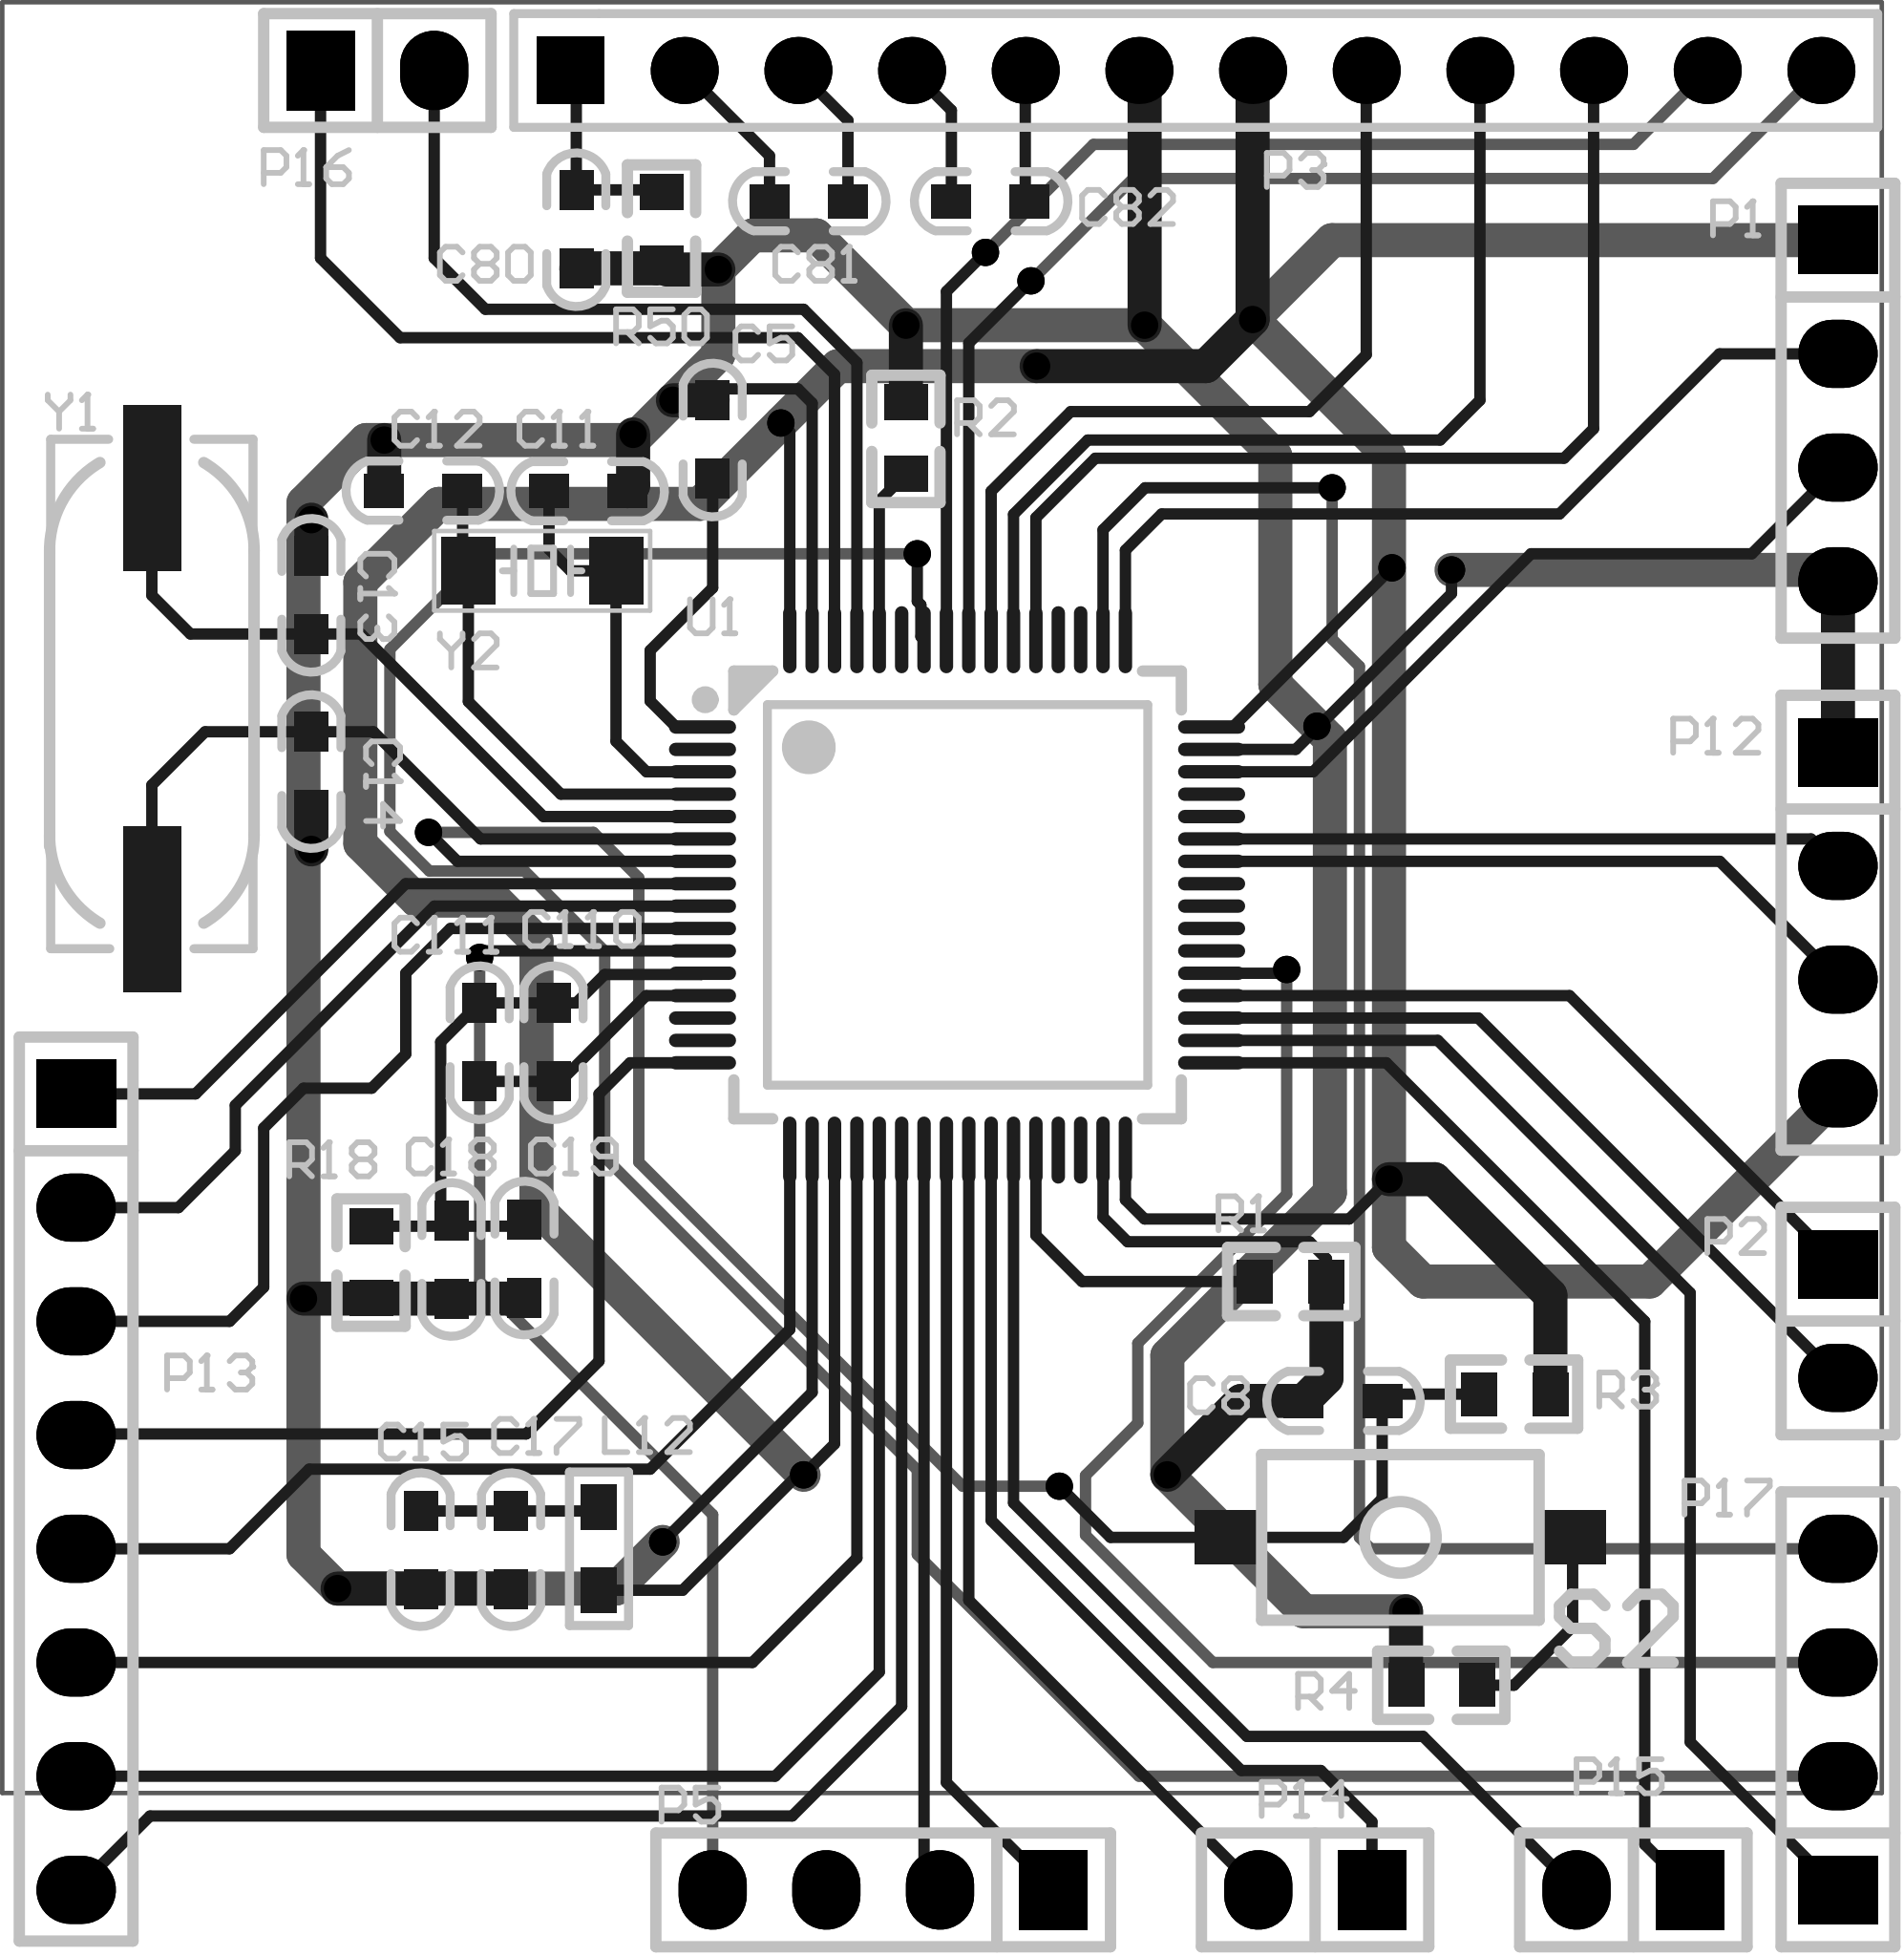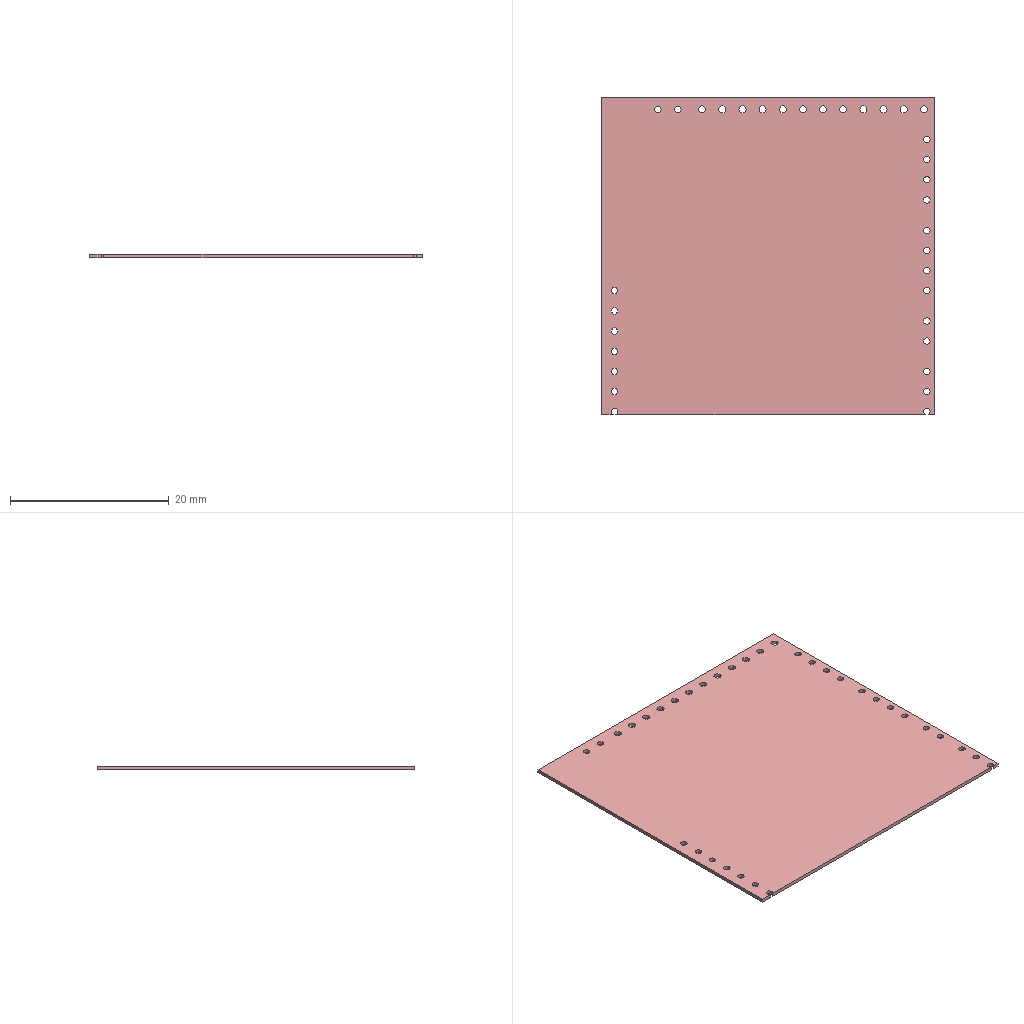Circuit board layout | Altium Designer | box 42 x 40 x 0.5 mm
Layer stack:
# Altium Designer layer stack of  (unit mm; dielectric type: 0 none, 1 core, 2 prepreg, 3 surface material)
index,name,kind,layer,copper_thickness_mm,dielectric_type,dielectric_thickness_mm,dielectric_material,dielectric_constant
0,Top Paste Mask Layer,other,,,,,,
1,Top Silkscreen Layer,other,,,,,,
2,Top Solder Mask Layer,dielectric,,,3,0.0356,FR-4,4.8
3,Top Layer,copper,Top Layer,0.0356,,,,
4,Substrate1,dielectric,,,3,0.32,FR-4,4.8
5,Bottom Layer,copper,Bottom Layer,0.0356,,,,
6,Bottom Solder Mask Layer,dielectric,,,3,0.0356,FR-4,4.8
7,Bottom Silkscreen Layer,other,,,,,,
8,Bottom Paste Mask Layer,other,,,,,,
# drill layer pairs: low layer,high layer
drill_pair,Top Layer,Bottom Layer
Part placement:
Designator,Comment,Layer,Footprint,Center-X(mm),Center-Y(mm),Rotation
S2,KEY,TopLayer,SWTP3.7X6,107.442,85.598,180
C5,1uF,TopLayer,C_0603,92.075,110.122,270
C8,104,TopLayer,C_0603,106.159,88.646,0
C11,20P,TopLayer,C_0603,89.294,108.966,180
C12,20P,TopLayer,C_0603,85.611,108.979,180
C13,20P,TopLayer,C_0603,83.107,106.654,270
C14,20P,TopLayer,C_0603,83.107,102.717,270
C15,1uF,TopLayer,C_0603,85.548,85.311,90
C17,0.01uF,TopLayer,C_0603,87.569,85.311,90
C18,1uF,TopLayer,C_0603,86.238,91.793,90
C19,0.01uF,TopLayer,C_0603,87.869,91.825,90
C80,330pF,TopLayer,C_0603,89.027,114.821,270
C81,2.2uF,TopLayer,C_0603,94.221,115.443,0
C82,2.2uF,TopLayer,C_0603,98.285,115.443,0
C110,0.1uF,TopLayer,C_0603,88.519,96.66,270
C111,0.01uF,TopLayer,C_0603,86.868,96.66,270
P1,Pin HDR1X4,TopLayer,Pin_HDR1X4/2.54mm-S,117.221,110.764,0
P2,Pin HDR1X2,TopLayer,Pin_HDR1X2/2.54mm-S,117.221,90.431,0
P3,Pin HDR1X12,TopLayer,Pin_HDR1X12/2.54mm-S,102.87,118.364,0
P5,Pin HDR1X4,TopLayer,Pin_HDR1X4/2.54mm-S,95.885,77.724,270
P12,Pin HDR1X4,TopLayer,Pin_HDR1X4/2.54mm-S,117.221,99.328,0
P13,Pin HDR1X8,TopLayer,Pin_HDR1X8/2.54mm-S,77.851,86.614,0
P14,Pin HDR1X2,TopLayer,Pin_HDR1X2/2.54mm-S,105.537,77.724,270
P15,Pin HDR1X2,TopLayer,Pin_HDR1X2/2.54mm-S,112.649,77.724,270
P16,Pin HDR1X2,TopLayer,Pin_HDR1X2/2.54mm-S,84.582,118.364,90
P17,Pin HDR1X4,TopLayer,Pin_HDR1X4/2.54mm-S,117.221,81.534,180
R1,10K,TopLayer,0603R,104.991,91.313,180
R2,10K,TopLayer,0603R,96.393,110.147,90
R3,10K,TopLayer,0603R,109.995,88.798,0
R4,330R,TopLayer,0603R,108.369,82.296,0
R18,0R,TopLayer,0603R,84.44,91.749,90
R50,3.3-10M,TopLayer,0603R,90.932,114.846,90
U1,STM32L152RBT6,TopLayer,LQFP-64_L10.0-W10.0-P0.50-LS12.0-BL,97.536,99.949,270
Y1,8MHz,TopLayer,XTAL_SMD49S,79.543,104.335,270
Y2,32.768kHz,TopLayer,OSC_3215-2P,88.265,107.188,180
L12,2uH,TopLayer,R_0603,89.535,85.344,270
Pad and via stacks:
# Altium Designer via and pad stacks of  (unit mm). Each distinct definition once, with the count of objects using it.
# via: kind,start_layer,end_layer,hole_mm,diameter_mm,mode(0 simple;1 top-mid-bottom;2 full stack),diameter_per_layer,count,example_net
# pad: kind,layer,hole_mm,hole_type(0 round;1 square;2 slot),plating,top_size,top_shape(1 round;2 rect;3 octagon;9 rounded rect),mid_size,bottom_size,mode,footprint,size_per_layer,count,example
pad,Top Layer,0,0,plated,1.5x1.2,2,1.5x1.2,1.5x1.2,0,SWTP3.7X6,,2,S2.2
pad,Top Layer,0,0,plated,0.889x0.762,2,0.889x0.762,0.889x0.762,0,C 0603,,30,C5.1
pad,Top Layer,0,0,plated,0.8x0.965,2,0.8x0.965,0.8x0.965,0,0603R,,12,R1.1
pad,Top Layer,0,0,plated,1.5x0.3,1,1.5x0.3,1.5x0.3,0,LQFP-64_L10.0-W10.0-P0.50-LS12.0-BL,,32,U1.64
pad,Top Layer,0,0,plated,0.3x1.5,1,0.3x1.5,0.3x1.5,0,LQFP-64_L10.0-W10.0-P0.50-LS12.0-BL,,32,U1.48
pad,Top Layer,0,0,plated,3.708x1.295,2,3.708x1.295,3.708x1.295,0,XTAL_SMD49S,,2,Y1.2
pad,Top Layer,0,0,plated,1.2x1.5,2,1.2x1.5,1.2x1.5,0,OSC 3215-2P,,2,Y2.2
pad,Top Layer,0,0,plated,1.016x0.8,2,1.016x0.8,1.016x0.8,0,R 0603,,2,L12.2
pad,Multi-Layer,0.8128,0,plated,1.524x1.778,2,1.524x1.778,1.524x1.778,0,Pin HDR1X4/2.54mm-S,,4,P1.1
pad,Multi-Layer,0.8128,0,plated,1.524x1.778,1,1.524x1.778,1.524x1.778,0,Pin HDR1X4/2.54mm-S,,12,P1.2
pad,Multi-Layer,0.8128,0,plated,1.524x1.778,2,1.524x1.778,1.524x1.778,0,Pin HDR1X2/2.54mm-S,,4,P2.1
pad,Multi-Layer,0.8128,0,plated,1.524x1.778,1,1.524x1.778,1.524x1.778,0,Pin HDR1X2/2.54mm-S,,4,P2.2
pad,Multi-Layer,0.9,0,plated,1.5x1.5,1,1.5x1.5,1.5x1.5,0,Pin HDR1X12/2.54mm-S,,11,P3.12
pad,Multi-Layer,0.9,0,plated,1.5x1.5,2,1.5x1.5,1.5x1.5,0,Pin HDR1X12/2.54mm-S,,1,P3.1
pad,Multi-Layer,0.8128,0,plated,1.524x1.778,1,1.524x1.778,1.524x1.778,0,Pin HDR1X8/2.54mm-S,,7,P13.8
pad,Multi-Layer,0.8128,0,plated,1.524x1.778,2,1.524x1.778,1.524x1.778,0,Pin HDR1X8/2.54mm-S,,1,P13.1
via,Top Layer,Bottom Layer,0.3048,0.61,0,,29,LCD_RST
Design rules, without the lines most boards share:
# Altium Designer design rules of  (exported by Altium Designer, unit mm)
# columns: name | kind | enabled | priority | scope1 | scope2 | descriptor | typed fields (field=value)
ComponentClearance_1 | 24 | enabled | 1 | All | All | Component Clearance Constraint ( Horizontal Gap = 10mil, Vertical Gap = 10mil ) (All),(All)  | gap=0.254
Clearance | 0 | enabled | 1 | All | All | Clearance Constraint (Gap=6mil) (All),(All) | gap=0.1524
Clearance_1 | 63 | enabled | 1 | All | All | Board Clearance Constraint (Gap=0mil) (All) |
creepage | 65 | enabled | 1 | All | All | Creepage Distance Constraint =(0mil) (All),(All) |
ComponentClearance | 52 | enabled | 1 | All | All | Hole To Hole Clearance (Gap=11.811mil) (All),(All) | gap=0.3
Width | 2 | enabled | 1 | All | All | Width Constraint (Min=8mil) (Max=30mil) (Preferred=10mil) (All) |
DiffPairsRouting | 51 | enabled | 1 | All | All | Differential Pairs Uncoupled Length using the Gap Constraints (Min=10mil) (Max=10mil) (Prefered=10mil)  and Width Constraints (Min=99999mil) (Max=0mil) (Prefered=0mil) (All) |
RoutingVias | 11 | enabled | 1 | All | All | Routing Via (MinHoleWidth=12mil) (MaxHoleWidth=15mil) (PreferredHoleWidth=15mil) (MinWidth=22mil) (MaxWidth=30mil) (PreferedWidth=30mil) (All) | via_min_hole=0.3048 via_max_hole=0.381 via_preferred_diameter=0.762 via_preferred_hole=0.381
PlaneConnect | 6 | enabled | 1 | All | All | Power Plane Connect Rule(Relief Connect )(Expansion=20mil) (Conductor Width=10mil) (Air Gap=10mil) (Entries=4) (All) | relief_conductor_width=0.254 relief_entries=4 relief_expansion=0.508
PolygonConnect | 20 | enabled | 1 | (InNet('TIM3_CH1') OR InNet('ADC_IN14')) | All | Polygon Connect Rule(Relief Connect )(Conductor Width=10mil) (Relief Angle=90 Angle) (Entries=4) (Air Gap Width=10mil) ((InNet('TIM3_CH1') OR InNet('ADC_IN14'))),(All) | connect_style(0=relief,1=direct,2=none)=0 relief_conductor_width=0.254 relief_entries=4
PasteMaskExpansion | 14 | enabled | 1 | All | All | Paste Mask Expansion (Expansion =0mil) (All) | expansion=0
SolderMaskExpansion | 13 | enabled | 1 | All | All | Solder Mask Expansion (Expansion =4mil) (All) | expansion=0.1016